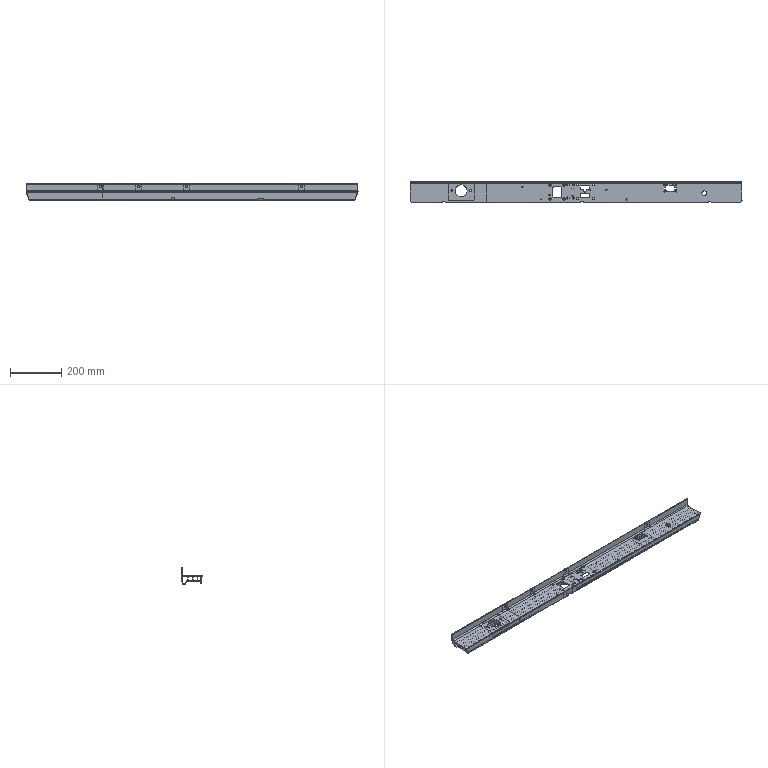NC program | NX | posted with a generic post | part box 1301 x 81.1 x 63 mm
Lines 5404 to 6411 of 19512:
(ZLEVEL_PROFILE_1 , TOOL : D8R0.5)
N10758 T08 M6
N10760 G54
N10762 G17 G0 G90 X413.988 Y35.772 B0. C0. S6000 M3
N10764 G43 Z30. H8
N10766 Z1.493
N10768 G94 G1 Z-0.007 F1000.
N10770 X415.22 Y36.791
N10772 G3 X415.359 Y37.166 R0.4
N10774 G1 X415.273 Y37.672 F2500.
N10776 Y39.829
N10778 X415.366 Y40.327
N10780 X415.253 Y40.366 Z-0.016
N10782 X415.164 Y39.863
N10784 Y37.637
N10786 X415.208 Y37.117
N10788 X415.148 Y37.097 Z-0.022
N10790 X415.104 Y37.082 Z-0.027
N10792 X415.063 Y37.599
N10794 Y39.901
N10796 X415.109 Y40.414
N10798 X415.01 Y40.446 Z-0.041
N10800 X414.964 Y39.935
N10802 Y37.565
N10804 X414.979 Y37.511
N10806 X415.014 Y37.054
N10808 X414.924 Y37.029 Z-0.058
N10810 X414.876 Y37.511
N10812 X414.864 Y37.533
N10814 Y39.967
N10816 X414.921 Y40.472
N10818 X414.818 Y40.502 Z-0.078
N10820 X414.765 Y39.998
N10822 Y37.501
N10824 X414.819 Y36.999
N10826 X414.701 Y36.964 Z-0.1
N10828 X414.667 Y37.47
N10830 Y40.03
N10832 X414.702 Y40.536
N10834 X414.653 Y40.549 Z-0.113
N10836 X414.609 Y40.561 Z-0.125
N10838 X414.572 Y40.06
N10840 Y37.441
N10842 X414.609 Y36.939
N10844 X414.555 Y36.925 Z-0.139
N10846 X414.521 Y36.916 Z-0.152
N10848 X414.478 Y37.413
N10850 Y40.087
N10852 X414.522 Y40.584
N10854 X414.459 Y40.6 Z-0.167
N10856 X414.427 Y40.608 Z-0.181
N10858 X414.387 Y40.112
N10860 Y37.388
N10862 X414.427 Y36.892
N10864 X414.367 Y36.877 Z-0.197
N10866 X414.325 Y36.866 Z-0.213
N10868 X414.298 Y37.364
N10870 Y40.136
N10872 X414.325 Y40.634
N10874 X414.275 Y40.646 Z-0.23
N10876 X414.23 Y40.656 Z-0.246
N10878 X414.21 Y40.158
N10880 Y37.342
N10882 X414.231 Y36.845
N10884 X414.182 Y36.836 Z-0.265
N10886 X414.144 Y36.829 Z-0.284
N10888 X414.119 Y37.322
N10890 Y40.178
N10892 X414.139 Y40.676
N10894 X414.086 Y40.687 Z-0.304
N10896 X414.038 Y40.697 Z-0.325
N10898 X414.028 Y40.198
N10900 Y37.302
N10902 X414.051 Y36.811
N10904 X413.992 Y36.8 Z-0.346
N10906 X413.954 Y36.793 Z-0.368
N10908 X413.937 Y37.285
N10910 Y40.215
N10912 X413.948 Y40.301
N10914 Y40.711
N10916 X413.9 Y40.717 Z-0.391
N10918 X413.858 Y40.723 Z-0.414
N10920 X413.848 Y40.228
N10922 Y37.272
N10924 X413.856 Y36.777
N10926 X413.813 Y36.775 Z-0.438
N10928 X413.772 Y36.773 Z-0.463
N10930 X413.76 Y37.261
N10932 Y40.239
N10934 X413.765 Y40.301
N10936 X413.775 Y40.727
N10938 X413.729 Y40.73 Z-0.488
N10940 X413.688 Y40.732 Z-0.514
N10942 X413.674 Y40.246
N10944 Y37.254
N10946 X413.684 Y36.768
N10948 X413.644 Y36.766 Z-0.54
N10950 X413.606 Y36.764 Z-0.567
N10952 X413.59 Y37.251
N10954 Y40.249
N10956 X413.611 Y40.736
N10958 X413.568 Y40.739 Z-0.595
N10960 X413.534 Y40.74 Z-0.623
N10962 X413.507 Y40.25
N10964 Y37.25
N10966 X413.526 Y36.759
N10968 X413.486 Y36.758 Z-0.652
N10970 X413.449 Y36.756 Z-0.681
N10972 X413.426 Y37.25
N10974 Y40.25
N10976 X413.455 Y40.746
N10978 X413.419 Y40.751 Z-0.711
N10980 X413.381 Y40.756 Z-0.741
N10982 X413.346 Y40.25
N10984 Y37.25
N10986 X413.38 Y36.755
N10988 X413.34 Y36.754 Z-0.772
N10990 X413.308 Y36.753 Z-0.803
N10992 X413.269 Y37.25
N10994 Y40.25
N10996 X413.27 Y40.301
N10998 X413.296 Y40.7
N11000 X413.304 Y40.767
N11002 X413.267 Y40.772 Z-0.836
N11004 X413.232 Y40.777 Z-0.868
N11006 X413.222 Y40.7
N11008 X413.193 Y40.25
N11010 Y37.25
N11012 X413.235 Y36.752
N11014 X413.189 Z-0.901
N11016 X413.159 Y36.751 Z-0.935
N11018 X413.119 Y37.25
N11020 Y40.25
N11022 X413.149 Y40.7
N11024 X413.16 Y40.787
N11026 X413.122 Y40.793 Z-0.969
N11028 X413.086 Y40.798 Z-1.003
N11030 X413.074 Y40.7
N11032 X413.047 Y40.25
N11034 Y37.25
N11036 X413.081 Y36.75
N11038 X413.046 Z-1.038
N11040 X413.016 Z-1.073
N11042 X412.978 Y37.25
N11044 Y40.25
N11046 X413.008 Y40.7
N11048 X413.019 Y40.793
N11050 X412.982 Y40.789 Z-1.11
N11052 X412.951 Y40.785 Z-1.146
N11054 X412.939 Y40.7
N11056 X412.91 Y40.25
N11058 Y37.25
N11060 X412.947 Y36.749
N11062 X412.91 Z-1.183
N11064 X412.878 Z-1.221
N11066 X412.843 Y37.25
N11068 Y40.25
N11070 X412.871 Y40.7
N11072 X412.882 Y40.778
N11074 X412.82 Y40.769 Z-1.297
N11076 X412.81 Y40.7
N11078 X412.785 Y40.301
N11080 X412.78 Y40.25
N11082 Y37.25
N11084 X412.818 Y36.75
N11086 X412.782 Z-1.337
N11088 X412.756 Z-1.376
N11090 X412.718 Y37.25
N11092 Y40.25
N11094 X412.748 Y40.7
N11096 X412.756 Y40.76
N11098 X412.691 Y40.751 Z-1.456
N11100 X412.681 Y40.658
N11102 X412.659 Y40.25
N11104 Y37.25
N11106 X412.693 Y36.751
N11108 X412.662 Z-1.497
N11110 X412.639 Z-1.538
N11112 X412.601 Y37.25
N11114 Y40.25
N11116 X412.607 Y40.301
N11118 X412.632 Y40.7
N11120 X412.637 Y40.75
N11122 X412.607 Z-1.58
N11124 X412.583 Y40.751 Z-1.621
N11126 X412.578 Y40.7
N11128 X412.552 Y40.301
N11130 X412.547 Y40.25
N11132 Y37.25
N11134 X412.586 Y36.75
N11136 X412.553 Y36.749 Z-1.664
N11138 X412.532 Z-1.706
N11140 X412.494 Y37.25
N11142 Y40.25
N11144 X412.496 Y40.301
N11146 X412.524 Y40.7
N11148 X412.529 Y40.752
N11150 X412.502 Z-1.749
N11152 X412.476 Z-1.793
N11154 X412.471 Y40.7
N11156 X412.449 Y40.301
N11158 X412.444 Y40.25
N11160 Y37.25
N11162 X412.478 Y36.749
N11164 X412.453 Z-1.837
N11166 X412.433 Z-1.881
N11168 X412.397 Y37.25
N11170 Y40.25
N11172 X412.405 Y40.301
N11174 X412.424 Y40.7
N11176 X412.429 Y40.752
N11178 X412.407 Z-1.925
N11180 X412.383 Z-1.97
N11182 X412.378 Y40.7
N11184 X412.359 Y40.301
N11186 X412.352 Y40.25
N11188 Y37.25
N11190 X412.386 Y36.749
N11192 X412.363 Z-2.015
N11194 X412.345 Z-2.06
N11196 X412.309 Y37.25
N11198 Y40.25
N11200 X412.314 Y40.301
N11202 X412.337 Y40.7
N11204 X412.342 Y40.751
N11206 X412.322 Z-2.106
N11208 X412.302 Y40.75 Z-2.152
N11210 G3 X412.27 Y40.25 R4.832
N11212 G1 Y37.25
N11214 G3 X412.304 Y36.75 R4.305
N11216 G1 X412.267 Y36.759 Z-2.245
N11218 X412.232 Y37.25
N11220 Y40.25
N11222 X412.239 Y40.301
N11224 X412.259 Y40.7
N11226 X412.266 Y40.75
N11228 X412.246 Y40.749 Z-2.292
N11230 X412.229 Z-2.339
N11232 X412.224 Y40.7
N11234 X412.205 Y40.301
N11236 X412.198 Y40.25
N11238 Y37.25
N11240 X412.231 Y36.777
N11242 X412.197 Y36.794 Z-2.433
N11244 X412.166 Y37.25
N11246 Y40.25
N11248 X412.171 Y40.301
N11250 X412.193 Y40.7
N11252 X412.197 Y40.747
N11254 X412.184 Y40.746 Z-2.481
N11256 X412.168 Y40.745 Z-2.529
N11258 X412.138 Y40.301
N11260 X412.137 Y40.25
N11262 Y37.25
N11264 G3 X412.167 Y36.811 R4.906
N11266 G1 X412.138 Y36.83 Z-2.625
N11268 X412.111 Y37.25
N11270 Y40.25
N11272 X412.137 Y40.7
N11274 X412.14 Y40.744
N11276 X412.131 Y40.742 Z-2.674
N11278 X412.118 Y40.741 Z-2.723
N11280 X412.087 Y40.25
N11282 Y37.25
N11284 X412.113 Y36.849
N11286 X412.09 Y36.867 Z-2.82
N11288 G2 X412.066 Y37.25 R4.587
N11290 G1 Y40.25
N11292 X412.067 Y40.301
N11294 X412.095 Y40.737
N11296 X412.086 Y40.736 Z-2.87
N11298 X412.072 Y40.734 Z-2.919
N11300 X412.05 Y40.301
N11302 X412.048 Y40.25
N11304 Y37.25
N11306 X412.068 Y36.888
N11308 X412.049 Y36.908 Z-3.018
N11310 X412.033 Y37.25
N11312 Y40.25
N11314 X412.035 Y40.301
N11316 X412.056 Y40.731
N11318 X412.05 Y40.73 Z-3.067
N11320 X412.039 Y40.728 Z-3.117
N11322 X412.026 Y40.301
N11324 X412.021 Y40.25
N11326 Y37.25
N11328 X412.035 Y36.931
N11330 X412.024 Y36.952 Z-3.213
N11332 X412.011 Y37.25
N11334 Y40.25
N11336 X412.017 Y40.301
N11338 X412.028 Y40.725
N11340 X412.018 Y40.722 Z-3.308
N11342 X412.009 Y40.301
N11344 X412.005 Y40.25
N11346 Y37.25
N11348 X412.015 Y36.972
N11350 X412.005 Y36.992 Z-3.404
N11352 X412.001 Y37.25
N11354 Y40.25
N11356 X412.008 Y40.719
N11358 X412.001 Y40.717 Z-3.5
N11360 Y37.012
N11362 G2 X411.601 Y36.319 R0.8
N11364 G1 X410.505 Y35.686
N11366 Z-2.
N11368 G0 Z30.
N11370 X441.954 Y41.797
N11372 Z1.493
N11374 G1 Z-0.007 F1000.
N11376 X440.746 Y40.721
N11378 G3 X440.62 Y40.341 R0.4
N11380 G1 X440.726 Y39.829 F2500.
N11382 Y37.672
N11384 X440.674 Y37.114
N11386 X440.796 Y37.112 Z-0.016
N11388 X440.835 Y37.637
N11390 Y39.863
N11392 X440.735 Y40.373
N11394 X440.843 Y40.403 Z-0.022
N11396 X440.878 Y40.413 Z-0.027
N11398 X440.936 Y39.901
N11400 Y37.599
N11402 X440.898 Y37.087
N11404 X440.888 Y37.081
N11406 X440.983 Y37.057 Z-0.041
N11408 X441.02 Y37.511
N11410 X441.036 Y37.565
N11412 Y39.935
N11414 X440.981 Y40.443
N11416 X441.072 Y40.47 Z-0.058
N11418 X441.135 Y39.967
N11420 Y37.533
N11422 X441.124 Y37.511
N11424 X441.072 Y37.03
N11426 X441.177 Y36.999 Z-0.078
N11428 X441.234 Y37.501
N11430 Y39.998
N11432 X441.177 Y40.501
N11434 X441.246 Y40.521 Z-0.089
N11436 X441.297 Y40.536 Z-0.1
N11438 X441.332 Y40.03
N11440 Y37.47
N11442 X441.297 Y36.964
N11444 X441.348 Y36.949 Z-0.113
N11446 X441.391 Y36.938 Z-0.125
N11448 X441.428 Y37.44
N11450 Y40.06
N11452 X441.391 Y40.562
N11454 X441.445 Y40.576 Z-0.139
N11456 X441.478 Y40.585 Z-0.152
N11458 X441.521 Y40.087
N11460 Y37.413
N11462 X441.479 Y36.915
N11464 X441.543 Y36.898 Z-0.167
N11466 X441.574 Y36.891 Z-0.181
N11468 X441.612 Y37.388
N11470 Y40.112
N11472 X441.573 Y40.609
N11474 X441.634 Y40.625 Z-0.197
N11476 X441.675 Y40.636 Z-0.213
N11478 X441.701 Y40.136
N11480 Y37.364
N11482 X441.676 Y36.864
N11484 X441.727 Y36.853 Z-0.23
N11486 X441.768 Y36.843 Z-0.246
N11488 X441.79 Y37.342
N11490 Y40.158
N11492 X441.77 Y40.658
N11494 X441.819 Y40.668 Z-0.265
N11496 X441.86 Y40.677 Z-0.284
N11498 X441.88 Y40.179
N11500 Y37.321
N11502 X441.853 Y36.827
N11504 X441.913 Y36.815 Z-0.304
N11506 X441.946 Y36.809 Z-0.325
N11508 X441.972 Y37.303
N11510 Y40.197
N11512 X441.959 Y40.698
N11514 X442.009 Y40.706 Z-0.346
N11516 X442.051 Y40.713 Z-0.368
N11518 X442.052 Y40.301
N11520 X442.062 Y40.215
N11522 Y37.285
N11524 X442.045 Y36.79
N11526 X442.101 Y36.781 Z-0.391
N11528 X442.144 Y36.774 Z-0.414
N11530 X442.151 Y37.272
N11532 Y40.228
N11534 X442.143 Y40.726
N11536 X442.19 Y40.728 Z-0.438
N11538 X442.228 Y40.73 Z-0.463
N11540 X442.234 Y40.301
N11542 X442.239 Y40.239
N11544 Y37.261
N11546 X442.228 Y36.77
N11548 X442.274 Y36.768 Z-0.488
N11550 X442.316 Y36.766 Z-0.514
N11552 X442.325 Y37.254
N11554 Y40.246
N11556 X442.316 Y40.735
N11558 X442.359 Y40.737 Z-0.54
N11560 X442.393 Y40.739 Z-0.567
N11562 X442.406 Y40.301
N11564 X442.41 Y40.249
N11566 Y37.251
N11568 X442.392 Y36.761
N11570 X442.435 Y36.759 Z-0.595
N11572 X442.468 Y36.757 Z-0.623
N11574 X442.492 Y37.25
N11576 Y40.25
N11578 X442.472 Y40.743
N11580 X442.516 Y40.745 Z-0.652
N11582 X442.55 Y40.746 Z-0.681
N11584 X442.574 Y40.25
N11586 Y37.25
N11588 X442.544 Y36.752
N11590 X442.581 Y36.748 Z-0.711
N11592 X442.614 Y36.744 Z-0.741
N11594 X442.653 Y37.25
N11596 Y40.25
N11598 X442.623 Y40.747
N11600 X442.659 Z-0.772
N11602 X442.699 Y40.748 Z-0.803
N11604 X442.73 Y40.301
N11606 X442.731 Y40.25
N11608 Y37.25
N11610 X442.686 Y36.737
N11612 X442.733 Y36.732 Z-0.836
N11614 X442.76 Y36.729 Z-0.868
N11616 X442.806 Y37.25
N11618 Y40.25
N11620 X442.777 Y40.7
N11622 X442.772 Y40.748
N11624 X442.81 Z-0.901
N11626 X442.845 Z-0.935
N11628 X442.851 Y40.7
N11630 X442.88 Y40.25
N11632 Y37.25
N11634 X442.837 Y36.721
N11636 X442.878 Y36.715 Z-0.969
N11638 X442.914 Y36.71 Z-1.003
N11640 X442.952 Y37.25
N11642 Y40.25
N11644 X442.925 Y40.7
N11646 X442.92 Y40.748
N11648 X442.955 Y40.749 Z-1.038
N11650 X442.986 Z-1.073
N11652 X442.992 Y40.7
N11654 X443.022 Y40.25
N11656 Y37.25
N11658 X442.983 Y36.716
N11660 X443.019 Y36.719 Z-1.11
N11662 X443.05 Y36.722 Z-1.146
N11664 X443.09 Y37.25
N11666 Y40.25
N11668 X443.06 Y40.7
N11670 X443.054 Y40.75
N11672 X443.09 Z-1.183
N11674 X443.121 Y40.751 Z-1.221
N11676 X443.129 Y40.7
N11678 X443.156 Y40.25
N11680 Y37.25
N11682 X443.118 Y36.728
N11684 X443.152 Y36.732 Z-1.259
N11686 X443.181 Y36.735 Z-1.297
N11688 X443.22 Y37.25
N11690 Y40.25
N11692 X443.215 Y40.301
N11694 X443.189 Y40.7
N11696 X443.182 Y40.75
N11698 X443.218 Z-1.337
N11700 X443.245 Z-1.376
N11702 X443.251 Y40.7
N11704 X443.281 Y40.25
N11706 Y37.25
N11708 X443.243 Y36.742
N11710 X443.279 Y36.746 Z-1.416
N11712 X443.306 Y36.75 Z-1.456
N11714 X443.341 Y37.25
N11716 Y40.25
N11718 X443.318 Y40.658
N11720 X443.308 Y40.749
N11722 X443.338 Y40.75 Z-1.497
N11724 X443.363 Z-1.538
N11726 X443.368 Y40.7
N11728 X443.392 Y40.301
N11730 X443.398 Y40.25
N11732 Y37.25
N11734 X443.36 Y36.75
N11736 X443.393 Z-1.58
N11738 X443.413 Z-1.621
N11740 X443.453 Y37.25
N11742 Y40.25
N11744 X443.447 Y40.301
N11746 X443.421 Y40.7
N11748 X443.416 Y40.751
N11750 X443.446 Z-1.664
N11752 X443.47 Y40.752 Z-1.706
N11754 X443.475 Y40.7
N11756 X443.503 Y40.301
N11758 X443.505 Y40.25
N11760 Y37.25
N11762 X443.467 Y36.749
N11764 X443.497 Z-1.749
N11766 X443.521 Z-1.793
N11768 X443.555 Y37.25
N11770 Y40.25
N11772 X443.55 Y40.301
N11774 X443.528 Y40.7
N11776 X443.523 Y40.752
N11778 X443.546 Z-1.837
N11780 X443.57 Z-1.881
N11782 X443.575 Y40.7
N11784 X443.595 Y40.301
N11786 X443.602 Y40.25
N11788 Y37.25
N11790 X443.566 Y36.749
N11792 X443.592 Z-1.925
N11794 X443.613 Z-1.97
N11796 X443.647 Y37.25
N11798 Y40.25
N11800 X443.64 Y40.301
N11802 X443.621 Y40.7
N11804 X443.617 Y40.752
N11806 X443.636 Y40.751 Z-2.015
N11808 X443.657 Z-2.06
N11810 X443.662 Y40.7
N11812 X443.685 Y40.301
N11814 X443.69 Y40.25
N11816 Y37.25
N11818 X443.654 Y36.749
N11820 X443.677 Y36.75 Z-2.106
N11822 X443.696 Z-2.152
N11824 G3 X443.73 Y37.25 R4.61
N11826 G1 Y40.25
N11828 X443.727 Y40.301
N11830 X443.703 Y40.7
N11832 X443.698 Y40.75
N11834 X443.717 Z-2.198
N11836 X443.732 Y40.749 Z-2.245
N11838 X443.737 Y40.7
N11840 X443.761 Y40.301
N11842 X443.767 Y40.25
N11844 Y37.25
N11846 X443.732 Y36.759
N11848 X443.766 Y36.777 Z-2.339
N11850 X443.801 Y37.25
N11852 Y40.25
N11854 X443.795 Y40.301
N11856 X443.769 Y40.7
N11858 X443.765 Y40.748
N11860 X443.785 Y40.747 Z-2.386
N11862 X443.797 Y40.746 Z-2.433
N11864 X443.829 Y40.301
N11866 X443.833 Y40.25
N11868 Y37.25
N11870 X443.801 Y36.794
N11872 X443.833 Y36.811 Z-2.529
N11874 G3 X443.862 Y37.25 R5.729
N11876 G1 Y40.25
N11878 X443.861 Y40.301
N11880 X443.829 Y40.745
N11882 X443.843 Z-2.577
N11884 X443.858 Y40.744 Z-2.625
N11886 X443.862 Y40.7
N11888 X443.889 Y40.25
N11890 Y37.25
N11892 X443.86 Y36.83
N11894 X443.887 Y36.849 Z-2.723
N11896 X443.912 Y37.25
N11898 Y40.25
N11900 X443.91 Y40.301
N11902 X443.88 Y40.742
N11904 X443.893 Y40.74 Z-2.772
N11906 X443.902 Y40.739 Z-2.82
N11908 X443.932 Y40.301
N11910 X443.933 Y40.25
N11912 Y37.25
N11914 X443.913 Y36.868
N11916 X443.934 Y36.889 Z-2.919
N11918 X443.951 Y37.25
N11920 Y40.25
N11922 X443.949 Y40.301
N11924 X443.924 Y40.736
N11926 X443.941 Y40.732 Z-3.018
N11928 X443.965 Y40.301
N11930 X443.966 Y40.25
N11932 Y37.25
N11934 X443.953 Y36.91
N11936 X443.966 Y36.932 Z-3.117
N11938 X443.979 Y37.25
N11940 Y40.25
N11942 X443.973 Y40.301
N11944 X443.957 Y40.729
N11946 X443.969 Y40.725 Z-3.213
N11948 X443.982 Y40.301
N11950 X443.988 Y40.25
N11952 Y37.25
N11954 X443.975 Y36.952
N11956 X443.984 Y36.972 Z-3.308
N11958 X443.994 Y37.25
N11960 Y40.25
N11962 X443.99 Y40.301
N11964 X443.98 Y40.723
N11966 X443.991 Y40.72 Z-3.404
N11968 X443.998 Y40.25
N11970 Y37.25
N11972 X443.993 Y36.992
N11974 X443.998 Y37.012 Z-3.5
N11976 X443.999 Y37.511
N11978 X443.998 Y40.301
N11980 X443.997 Y40.716
N11982 G2 X444.394 Y41.41 R0.8
N11984 G1 X445.452 Y42.026
N11986 Z-2.
N11988 G0 Z30.
N11990 X-34.943 Y35.568
N11992 Z1.493
N11994 G1 Z-0.007 F1000.
N11996 X-33.919 Y36.416
N11998 G3 X-33.64 Y37.166 R0.8
N12000 G1 X-33.726 Y37.672 F2500.
N12002 Y39.829
N12004 X-33.603 Y40.5
N12006 X-33.72 Y40.473 Z-0.016
N12008 X-33.835 Y39.863
N12010 Y37.637
N12012 X-33.791 Y37.117
N12014 X-33.851 Y37.097 Z-0.022
N12016 X-33.895 Y37.082 Z-0.027
N12018 X-33.936 Y37.599
N12020 Y39.901
N12022 X-33.872 Y40.44
N12024 X-33.949 Y40.442 Z-0.034
N12026 X-33.981 Y40.443 Z-0.041
N12028 X-34.035 Y39.935
N12030 Y37.565
N12032 X-34.02 Y37.511
N12034 X-33.986 Y37.054
N12036 X-34.076 Y37.028 Z-0.058
N12038 X-34.124 Y37.511
N12040 X-34.135 Y37.533
N12042 Y39.967
N12044 X-34.072 Y40.47
N12046 X-34.177 Y40.501 Z-0.078
N12048 X-34.234 Y39.998
N12050 Y37.501
N12052 X-34.18 Y36.998
N12054 X-34.298 Y36.964 Z-0.1
N12056 X-34.332 Y37.47
N12058 Y40.03
N12060 X-34.297 Y40.536
N12062 X-34.348 Y40.551 Z-0.113
N12064 X-34.391 Y40.562 Z-0.125
N12066 X-34.428 Y40.06
N12068 Y37.441
N12070 X-34.39 Y36.938
N12072 X-34.444 Y36.925 Z-0.139
N12074 X-34.478 Y36.916 Z-0.152
N12076 X-34.521 Y37.413
N12078 Y40.087
N12080 X-34.479 Y40.585
N12082 X-34.543 Y40.602 Z-0.167
N12084 X-34.574 Y40.61 Z-0.181
N12086 X-34.612 Y40.112
N12088 Y37.388
N12090 X-34.572 Y36.892
N12092 X-34.631 Y36.877 Z-0.197
N12094 X-34.673 Y36.867 Z-0.213
N12096 X-34.701 Y37.364
N12098 Y40.136
N12100 X-34.676 Y40.636
N12102 X-34.726 Y40.648 Z-0.23
N12104 X-34.77 Y40.658 Z-0.246
N12106 X-34.789 Y40.158
N12108 Y37.342
N12110 X-34.767 Y36.845
N12112 X-34.816 Y36.836 Z-0.265
N12114 X-34.855 Y36.829 Z-0.284
N12116 X-34.88 Y37.322
N12118 Y40.179
N12120 X-34.861 Y40.677
N12122 X-34.915 Y40.688 Z-0.304
N12124 X-34.961 Y40.698 Z-0.325
N12126 X-34.972 Y40.197
N12128 Y37.302
N12130 X-34.948 Y36.812
N12132 X-35.007 Y36.8 Z-0.346
N12134 X-35.045 Y36.793 Z-0.368
N12136 X-35.062 Y37.285
N12138 Y40.215
N12140 X-35.051 Y40.301
N12142 Y40.713
N12144 X-35.101 Y40.72 Z-0.391
N12146 X-35.143 Y40.726 Z-0.414
N12148 X-35.151 Y40.228
N12150 Y37.272
N12152 X-35.143 Y36.777
N12154 X-35.186 Y36.775 Z-0.438
N12156 X-35.227 Y36.773 Z-0.463
N12158 X-35.239 Y37.261
N12160 Y40.239
N12162 X-35.234 Y40.301
N12164 X-35.227 Y40.73
N12166 X-35.274 Y40.733 Z-0.488
N12168 X-35.315 Y40.735 Z-0.514
N12170 X-35.325 Y40.246
N12172 Y37.254
N12174 X-35.315 Y36.768
N12176 X-35.355 Y36.766 Z-0.54
N12178 X-35.393 Y36.764 Z-0.567
N12180 X-35.409 Y37.251
N12182 Y40.249
N12184 X-35.405 Y40.301
N12186 X-35.39 Y40.739
N12188 X-35.435 Y40.741 Z-0.595
N12190 X-35.467 Y40.743 Z-0.623
N12192 X-35.492 Y40.25
N12194 Y37.25
N12196 X-35.473 Y36.759
N12198 X-35.514 Y36.758 Z-0.652
N12200 X-35.55 Y36.756 Z-0.681
N12202 X-35.573 Y37.25
N12204 Y40.25
N12206 X-35.545 Y40.749
N12208 X-35.58 Y40.753 Z-0.711
N12210 X-35.619 Y40.758 Z-0.741
N12212 X-35.653 Y40.25
N12214 Y37.25
N12216 X-35.619 Y36.755
N12218 X-35.659 Y36.754 Z-0.772
N12220 X-35.691 Y36.753 Z-0.803
N12222 X-35.73 Y37.25
N12224 Y40.25
N12226 Y40.301
N12228 X-35.703 Y40.7
N12230 X-35.695 Y40.768
N12232 X-35.732 Y40.773 Z-0.836
N12234 X-35.767 Y40.778 Z-0.868
N12236 X-35.777 Y40.7
N12238 X-35.806 Y40.25
N12240 Y37.25
N12242 X-35.764 Y36.752
N12244 X-35.81 Z-0.901
N12246 X-35.84 Y36.751 Z-0.935
N12248 X-35.88 Y37.25
N12250 Y40.25
N12252 X-35.85 Y40.7
N12254 X-35.839 Y40.787
N12256 X-35.877 Y40.792 Z-0.969
N12258 X-35.913 Y40.797 Z-1.003
N12260 X-35.925 Y40.7
N12262 X-35.952 Y40.25
N12264 Y37.25
N12266 X-35.918 Y36.75
N12268 X-35.954 Z-1.038
N12270 X-35.984 Z-1.073
N12272 X-36.021 Y37.25
N12274 Y40.25
N12276 X-35.991 Y40.7
N12278 X-35.981 Y40.792
N12280 X-36.017 Y40.788 Z-1.11
N12282 X-36.048 Y40.785 Z-1.146
N12284 X-36.06 Y40.7
N12286 X-36.09 Y40.25
N12288 Y37.25
N12290 X-36.052 Y36.749
N12292 X-36.09 Z-1.183
N12294 X-36.121 Z-1.221
N12296 X-36.156 Y37.25
N12298 Y40.25
N12300 X-36.129 Y40.7
N12302 X-36.117 Y40.778
N12304 X-36.179 Y40.769 Z-1.297
N12306 X-36.189 Y40.7
N12308 X-36.215 Y40.301
N12310 X-36.219 Y40.25
N12312 Y37.25
N12314 X-36.181 Y36.75
N12316 X-36.218 Z-1.337
N12318 X-36.243 Z-1.376
N12320 X-36.281 Y37.25
N12322 Y40.25
N12324 X-36.251 Y40.7
N12326 X-36.243 Y40.76
N12328 X-36.308 Y40.751 Z-1.456
N12330 X-36.318 Y40.658
N12332 X-36.341 Y40.25
N12334 Y37.25
N12336 X-36.306 Y36.751
N12338 X-36.338 Z-1.497
N12340 X-36.36 Z-1.538
N12342 X-36.398 Y37.25
N12344 Y40.25
N12346 X-36.392 Y40.301
N12348 X-36.367 Y40.7
N12350 X-36.363 Y40.75
N12352 X-36.392 Z-1.58
N12354 X-36.416 Y40.751 Z-1.621
N12356 X-36.421 Y40.7
N12358 X-36.447 Y40.301
N12360 X-36.452 Y40.25
N12362 Y37.25
N12364 X-36.413 Y36.75
N12366 X-36.446 Y36.749 Z-1.664
N12368 X-36.467 Z-1.706
N12370 X-36.505 Y37.25
N12372 Y40.25
N12374 X-36.503 Y40.301
N12376 X-36.475 Y40.7
N12378 X-36.47 Y40.752
N12380 X-36.497 Z-1.749
N12382 X-36.523 Z-1.793
N12384 X-36.528 Y40.7
N12386 X-36.55 Y40.301
N12388 X-36.555 Y40.25
N12390 Y37.25
N12392 X-36.521 Y36.749
N12394 X-36.546 Z-1.837
N12396 X-36.566 Z-1.881
N12398 X-36.602 Y37.25
N12400 Y40.25
N12402 X-36.595 Y40.301
N12404 X-36.575 Y40.7
N12406 X-36.57 Y40.752
N12408 X-36.592 Z-1.925
N12410 X-36.616 Z-1.97
N12412 X-36.621 Y40.7
N12414 X-36.64 Y40.301
N12416 X-36.647 Y40.25
N12418 Y37.25
N12420 X-36.613 Y36.749
N12422 X-36.636 Z-2.015
N12424 X-36.654 Z-2.06
N12426 X-36.69 Y37.25
N12428 Y40.25
N12430 X-36.685 Y40.301
N12432 X-36.662 Y40.7
N12434 X-36.657 Y40.751
N12436 X-36.677 Z-2.106
N12438 X-36.698 Y40.75 Z-2.152
N12440 G3 X-36.729 Y40.25 R4.833
N12442 G1 Y37.25
N12444 G3 X-36.695 Y36.75 R4.305
N12446 G1 X-36.733 Y36.759 Z-2.245
N12448 X-36.767 Y37.25
N12450 Y40.25
N12452 X-36.761 Y40.301
N12454 X-36.74 Y40.7
N12456 X-36.734 Y40.75
N12458 X-36.751 Y40.749 Z-2.292
N12460 X-36.77 Z-2.339
N12462 X-36.775 Y40.7
N12464 X-36.794 Y40.301
N12466 X-36.801 Y40.25
N12468 Y37.25
N12470 X-36.768 Y36.777
N12472 X-36.802 Y36.794 Z-2.433
N12474 X-36.833 Y37.25
N12476 Y40.25
N12478 X-36.828 Y40.301
N12480 X-36.806 Y40.7
N12482 X-36.802 Y40.747
N12484 X-36.815 Y40.746 Z-2.481
N12486 X-36.831 Y40.745 Z-2.529
N12488 X-36.861 Y40.301
N12490 X-36.862 Y40.25
N12492 Y37.25
N12494 G3 X-36.832 Y36.811 R4.906
N12496 G1 X-36.861 Y36.83 Z-2.625
N12498 X-36.888 Y37.25
N12500 Y40.25
N12502 X-36.862 Y40.7
N12504 X-36.859 Y40.744
N12506 X-36.868 Y40.742 Z-2.674
N12508 X-36.881 Y40.741 Z-2.723
N12510 X-36.912 Y40.25
N12512 Y37.25
N12514 X-36.886 Y36.849
N12516 X-36.91 Y36.867 Z-2.82
N12518 G2 X-36.933 Y37.25 R4.587
N12520 G1 Y40.25
N12522 X-36.932 Y40.301
N12524 X-36.904 Y40.737
N12526 X-36.913 Y40.736 Z-2.87
N12528 X-36.927 Y40.734 Z-2.919
N12530 X-36.949 Y40.301
N12532 X-36.951 Y40.25
N12534 Y37.25
N12536 X-36.931 Y36.888
N12538 X-36.95 Y36.908 Z-3.018
N12540 X-36.966 Y37.25
N12542 Y40.25
N12544 X-36.964 Y40.301
N12546 X-36.943 Y40.731
N12548 X-36.949 Y40.73 Z-3.067
N12550 X-36.96 Y40.728 Z-3.117
N12552 X-36.973 Y40.301
N12554 X-36.978 Y40.25
N12556 Y37.25
N12558 X-36.964 Y36.931
N12560 X-36.975 Y36.952 Z-3.213
N12562 X-36.988 Y37.25
N12564 Y40.25
N12566 X-36.982 Y40.301
N12568 X-36.971 Y40.725
N12570 X-36.981 Y40.722 Z-3.308
N12572 X-36.99 Y40.301
N12574 X-36.994 Y40.25
N12576 Y37.25
N12578 X-36.984 Y36.972
N12580 X-36.994 Y36.992 Z-3.404
N12582 X-36.998 Y37.25
N12584 Y40.25
N12586 X-36.991 Y40.719
N12588 X-36.998 Y40.717 Z-3.5
N12590 Y37.012
N12592 G2 X-37.398 Y36.319 R0.8
N12594 G1 X-38.494 Y35.686
N12596 Z-2.
N12598 G0 Z30.
N12600 X-7.044 Y41.798
N12602 Z1.493
N12604 G1 Z-0.007 F1000.
N12606 X-8.254 Y40.721
N12608 G3 X-8.379 Y40.341 R0.4
N12610 G1 X-8.273 Y39.829 F2500.
N12612 Y37.672
N12614 X-8.325 Y37.114
N12616 X-8.203 Y37.112 Z-0.016
N12618 X-8.164 Y37.637
N12620 Y39.863
N12622 X-8.264 Y40.373
N12624 X-8.156 Y40.403 Z-0.022
N12626 X-8.121 Y40.413 Z-0.027
N12628 X-8.063 Y39.901
N12630 Y37.599
N12632 X-8.101 Y37.087
N12634 X-8.111 Y37.081
N12636 X-8.016 Y37.057 Z-0.041
N12638 X-7.979 Y37.511
N12640 X-7.964 Y37.565
N12642 Y39.935
N12644 X-8.018 Y40.443
N12646 X-7.927 Y40.47 Z-0.058
N12648 X-7.864 Y39.967
N12650 Y37.533
N12652 X-7.876 Y37.511
N12654 X-7.927 Y37.03
N12656 X-7.822 Y36.999 Z-0.078
N12658 X-7.765 Y37.501
N12660 Y39.998
N12662 X-7.822 Y40.501
N12664 X-7.753 Y40.521 Z-0.089
N12666 X-7.702 Y40.536 Z-0.1
N12668 X-7.667 Y40.03
N12670 Y37.47
N12672 X-7.702 Y36.964
N12674 X-7.608 Y36.938 Z-0.125
N12676 X-7.571 Y37.44
N12678 Y40.06
N12680 X-7.608 Y40.562
N12682 X-7.553 Y40.577 Z-0.139
N12684 X-7.52 Y40.585 Z-0.152
N12686 X-7.478 Y40.087
N12688 Y37.413
N12690 X-7.52 Y36.915
N12692 X-7.455 Y36.898 Z-0.167
N12694 X-7.425 Y36.89 Z-0.181
N12696 X-7.387 Y37.388
N12698 Y40.112
N12700 X-7.425 Y40.61
N12702 X-7.364 Y40.625 Z-0.197
N12704 X-7.323 Y40.636 Z-0.213
N12706 X-7.298 Y40.136
N12708 Y37.364
N12710 X-7.323 Y36.864
N12712 X-7.272 Y36.853 Z-0.23
N12714 X-7.231 Y36.843 Z-0.246
N12716 X-7.21 Y37.342
N12718 Y40.158
N12720 X-7.229 Y40.658
N12722 X-7.179 Y40.669 Z-0.265
N12724 X-7.139 Y40.677 Z-0.284
N12726 X-7.119 Y40.179
N12728 Y37.321
N12730 X-7.146 Y36.827
N12732 X-7.086 Y36.815 Z-0.304
N12734 X-7.053 Y36.809 Z-0.325
N12736 X-7.027 Y37.303
N12738 Y40.197
N12740 X-7.04 Y40.698
N12742 X-6.99 Y40.706 Z-0.346
N12744 X-6.948 Y40.713 Z-0.368
N12746 X-6.947 Y40.301
N12748 X-6.937 Y40.215
N12750 Y37.285
N12752 X-6.954 Y36.79
N12754 X-6.899 Y36.781 Z-0.391
N12756 X-6.855 Y36.774 Z-0.414
N12758 X-6.848 Y37.272
N12760 Y40.228
N12762 X-6.856 Y40.726
N12764 X-6.81 Y40.728 Z-0.438
N12766 X-6.771 Y40.73 Z-0.463